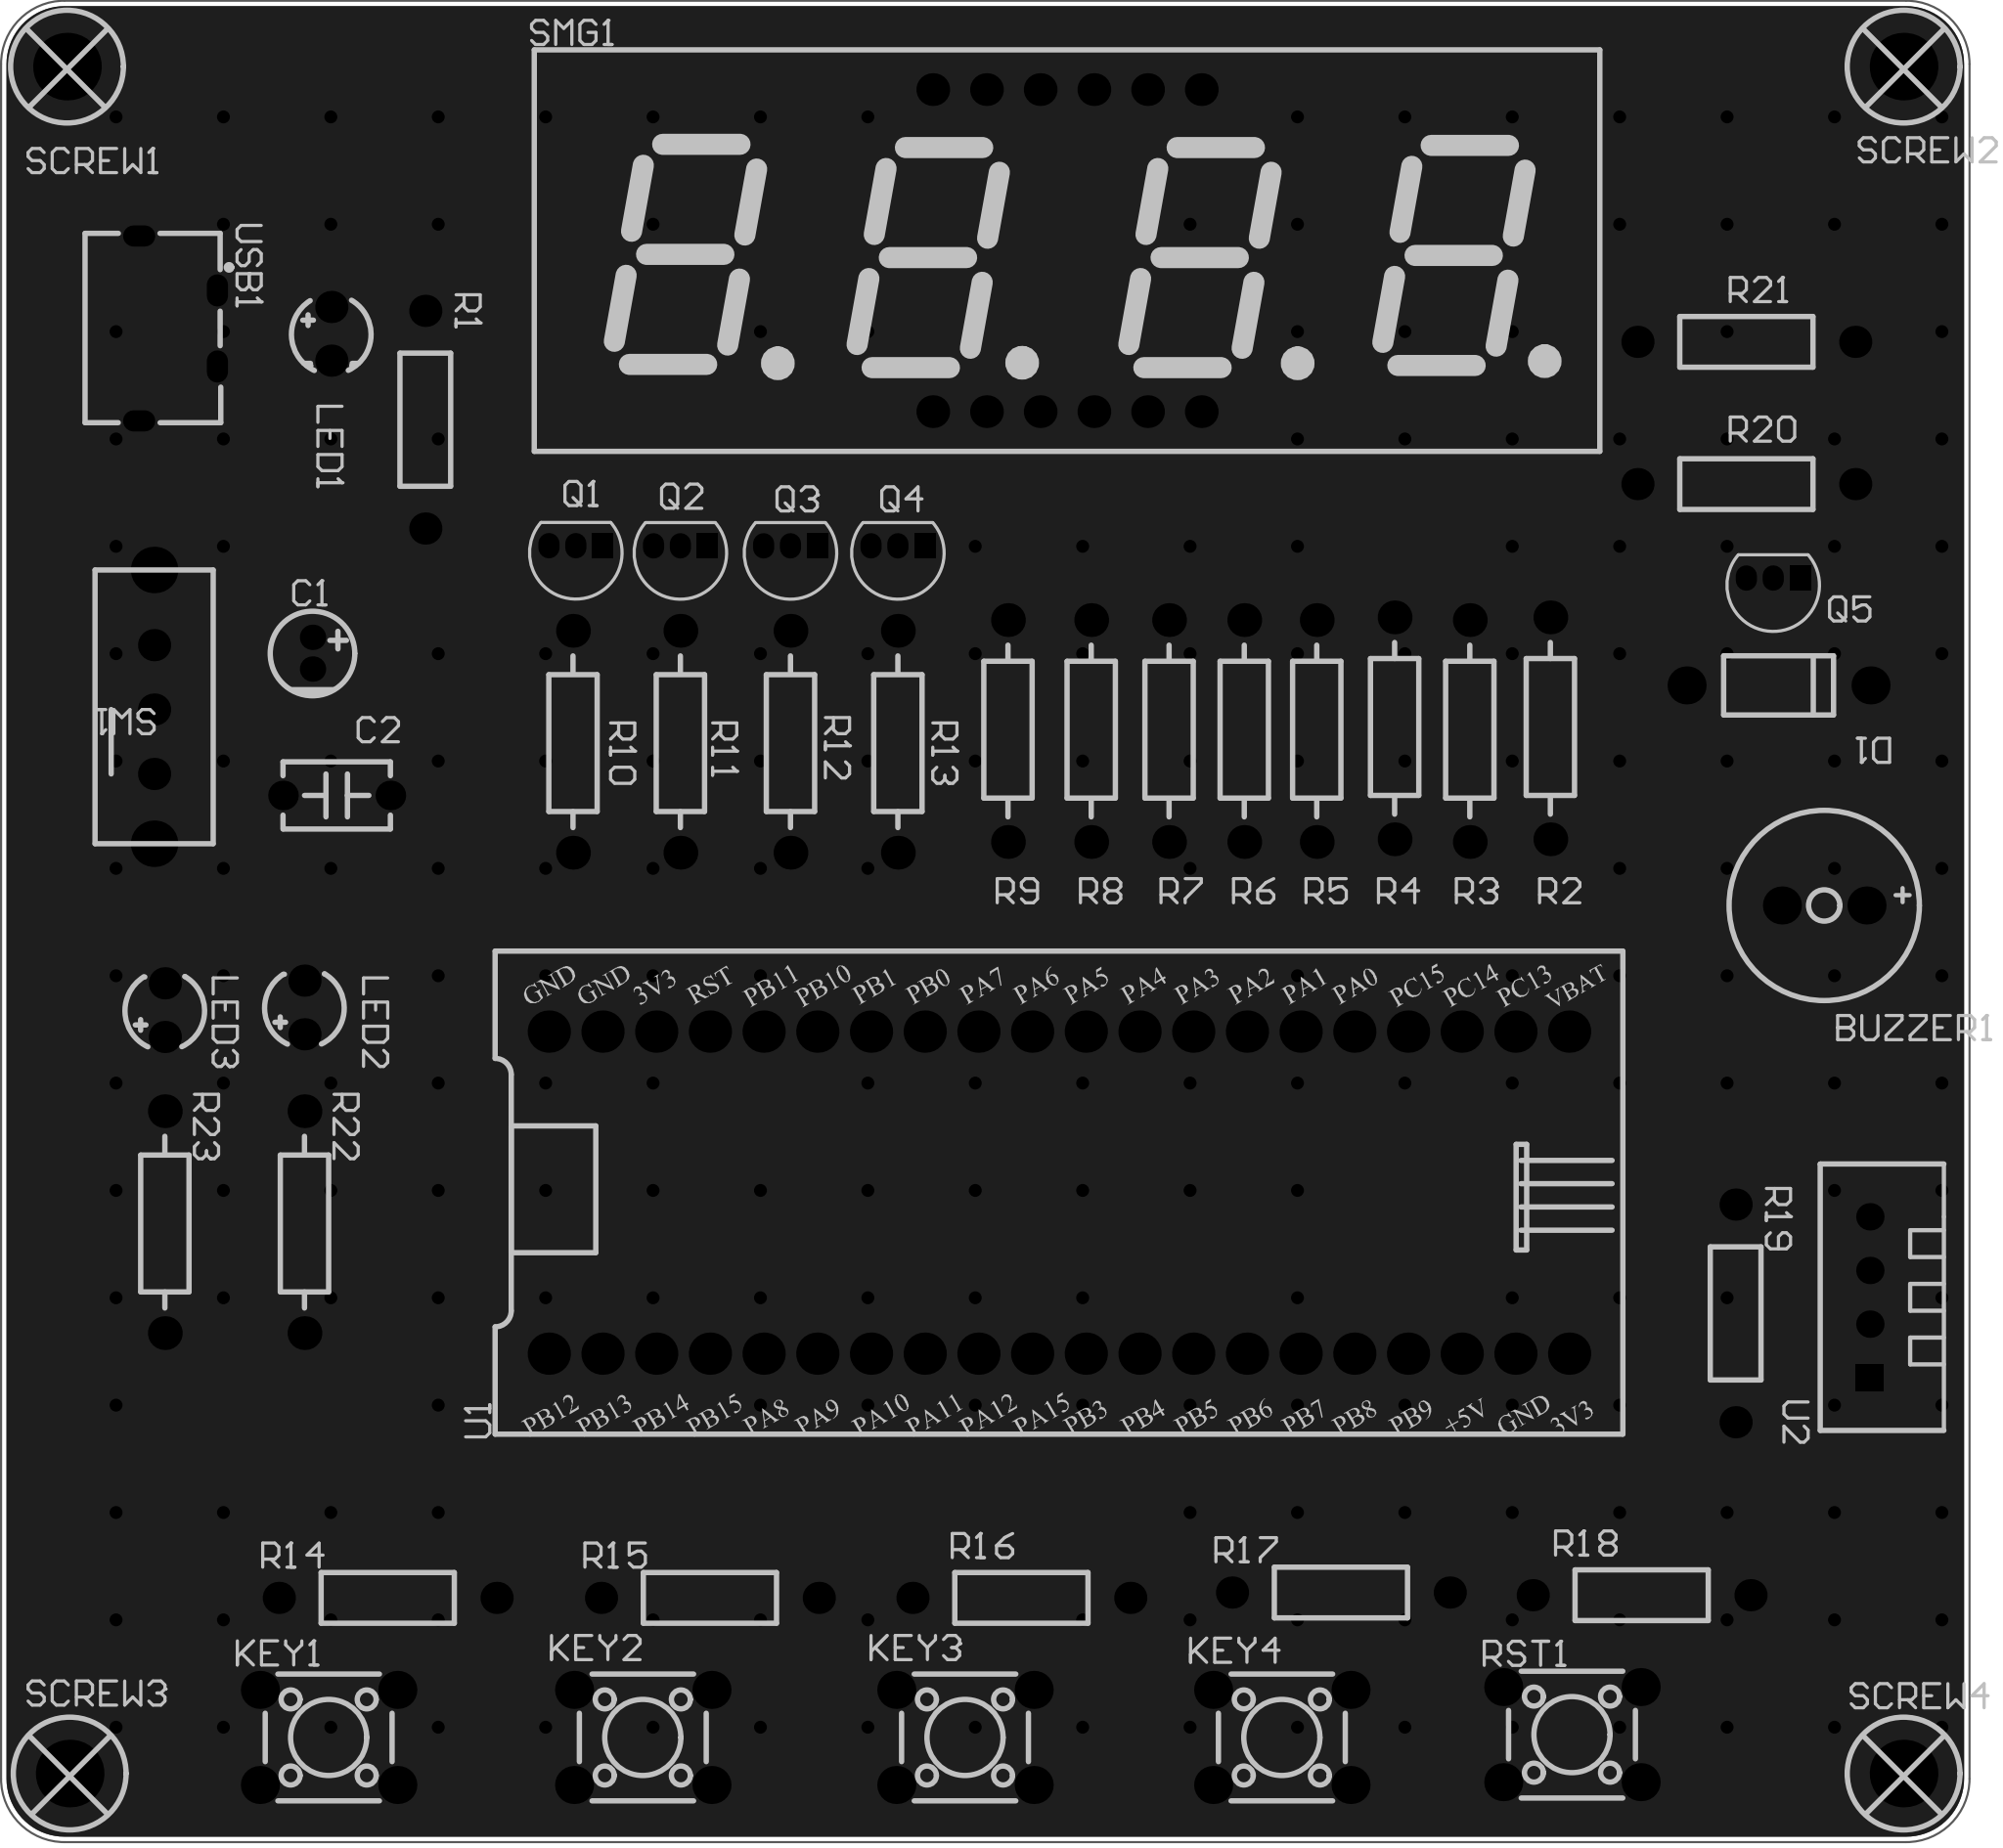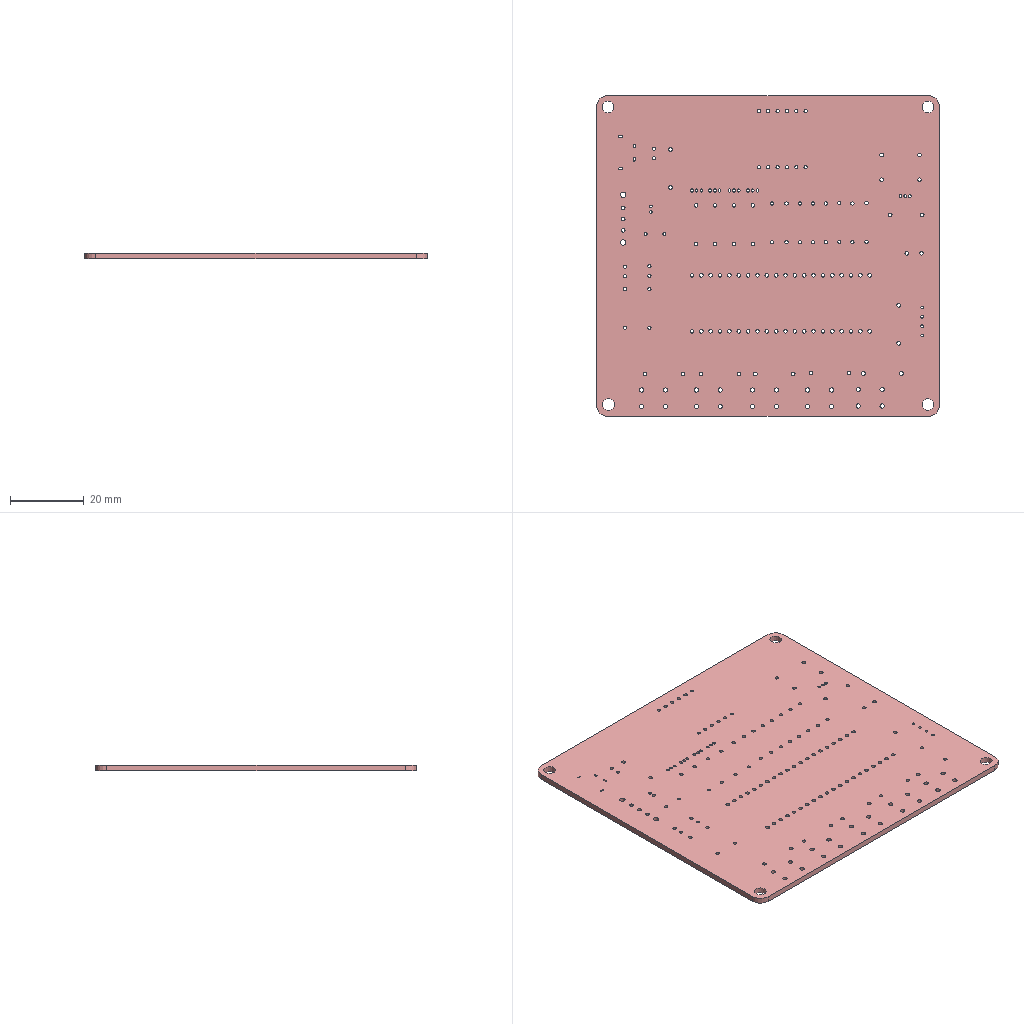Circuit board layout | Altium Designer | box 93.1 x 87.1 x 1.6 mm
Layer stack:
# Altium Designer layer stack of  (unit mm; dielectric type: 0 none, 1 core, 2 prepreg, 3 surface material)
index,name,kind,layer,copper_thickness_mm,dielectric_type,dielectric_thickness_mm,dielectric_material,dielectric_constant
0,Top Paste Mask Layer,other,,,,,,
1,Top Silkscreen Layer,other,,,,,,
2,Top Solder Mask Layer,dielectric,,,3,0.01,,3.3
3,Top Layer,copper,Top Layer,0.035,,,,
4,Dielectric1,dielectric,,,3,1.51,FR4,4.5
5,Bottom Layer,copper,Bottom Layer,0.035,,,,
6,Bottom Solder Mask Layer,dielectric,,,3,0.01,,3.3
7,Bottom Silkscreen Layer,other,,,,,,
8,Bottom Paste Mask Layer,other,,,,,,
# drill layer pairs: low layer,high layer
drill_pair,Top Layer,Bottom Layer
Part placement:
Designator,Comment,Layer,Footprint,Center-X(mm),Center-Y(mm),Rotation
BUZZER1,2.7kHz,TopLayer,BUZ-TH_BD9.0-P4.00-D0.6-FD,173.99,133.604,180
C1,10uF,TopLayer,CAP-TH_BD4.0-P1.50-D0.8-FD,102.489,145.542,270
C2,100nF,TopLayer,CAP-TH_L5.0-W2.5-P5.08-D0.7,103.632,138.811,180
D1,1N5819,TopLayer,DO-41_BD2.4-L4.7-P8.70-D0.9-RD,171.831,144.018,180
KEY1,TS-1002-07026,TopLayer,SW-TH_4P-L6.0-W6.0-P4.50-LS6.5,103.251,94.234,0
KEY2,TS-1002-07026,TopLayer,SW-TH_4P-L6.0-W6.0-P4.50-LS6.5,118.11,94.234,0
KEY3,TS-1002-07026,TopLayer,SW-TH_4P-L6.0-W6.0-P4.50-LS6.5,133.35,94.234,0
KEY4,TS-1002-07026,TopLayer,SW-TH_4P-L6.0-W6.0-P4.50-LS6.5,148.336,94.234,0
LED1,XL-302SURD,TopLayer,LED-TH_BD3.8-P2.54-RD,103.378,160.655,90
LED2,XL-302UGD,TopLayer,LED-TH_BD3.8-P2.54-FD_GREEN,102.108,128.778,90
LED3,XL-302UGD,TopLayer,LED-TH_BD3.8-P2.54-FD_GREEN,95.504,128.651,90
Q1,S8050,TopLayer,TO-92-3_L4.5-W3.5-P1.27-L,114.942,150.629,180
Q2,S8050,TopLayer,TO-92-3_L4.5-W3.5-P1.27-L,119.888,150.622,180
Q3,S8050,TopLayer,TO-92-3_L4.5-W3.5-P1.27-L,125.095,150.622,180
Q4,S8050,TopLayer,TO-92-3_L4.5-W3.5-P1.27-L,130.175,150.622,180
Q5,S8050,TopLayer,TO-92-3_L4.5-W3.5-P1.27-L,171.577,149.098,180
R1,10kΩ,TopLayer,RES-TH_BD2.4-L6.3-P10.30-D0.6,107.823,156.591,270
R2,330Ω,TopLayer,RES-TH_BD2.2-L6.5-P10.50-D0.6,161.036,141.986,90
R3,330Ω,TopLayer,RES-TH_BD2.2-L6.5-P10.50-D0.6,157.226,141.859,90
R4,330Ω,TopLayer,RES-TH_BD2.2-L6.5-P10.50-D0.6,153.67,141.986,90
R5,330Ω,TopLayer,RES-TH_BD2.2-L6.5-P10.50-D0.6,149.987,141.859,90
R6,330Ω,TopLayer,RES-TH_BD2.2-L6.5-P10.50-D0.6,146.558,141.859,90
R7,330Ω,TopLayer,RES-TH_BD2.2-L6.5-P10.50-D0.6,143.002,141.859,90
R8,330Ω,TopLayer,RES-TH_BD2.2-L6.5-P10.50-D0.6,139.319,141.859,90
R9,330Ω,TopLayer,RES-TH_BD2.2-L6.5-P10.50-D0.6,135.382,141.859,90
R10,1kΩ,TopLayer,RES-TH_BD2.2-L6.5-P10.50-D0.6,114.808,141.351,270
R11,1kΩ,TopLayer,RES-TH_BD2.2-L6.5-P10.50-D0.6,119.888,141.351,270
R12,1kΩ,TopLayer,RES-TH_BD2.2-L6.5-P10.50-D0.6,125.095,141.351,270
R13,1kΩ,TopLayer,RES-TH_BD2.2-L6.5-P10.50-D0.6,130.175,141.351,270
R14,10kΩ,TopLayer,RES-TH_BD2.4-L6.3-P10.30-D0.6,106.045,100.838,0
R15,10kΩ,TopLayer,RES-TH_BD2.4-L6.3-P10.30-D0.6,121.285,100.838,0
R16,10kΩ,TopLayer,RES-TH_BD2.4-L6.3-P10.30-D0.6,136.017,100.838,180
R17,10kΩ,TopLayer,RES-TH_BD2.4-L6.3-P10.30-D0.6,151.13,101.092,0
R18,10kΩ,TopLayer,RES-TH_BD2.4-L6.3-P10.30-D0.6,165.354,100.965,180
R19,10kΩ,TopLayer,RES-TH_BD2.4-L6.3-P10.30-D0.6,169.799,114.3,270
R20,10kΩ,TopLayer,RES-TH_BD2.4-L6.3-P10.30-D0.6,170.307,153.543,180
R21,10kΩ,TopLayer,RES-TH_BD2.4-L6.3-P10.30-D0.6,170.307,160.274,0
R22,1kΩ,TopLayer,RES-TH_BD2.2-L6.5-P10.50-D0.6,102.108,118.618,270
R23,1kΩ,TopLayer,RES-TH_BD2.2-L6.5-P10.50-D0.6,95.504,118.618,270
RST1,TS-1002-07026,TopLayer,SW-TH_4P-L6.0-W6.0-P4.50-LS6.5,162.059,94.368,0
SCREW1,,TopLayer,M3螺丝,90.876,173.298,0
SCREW2,,TopLayer,M3螺丝,177.744,173.298,0
SCREW3,,TopLayer,M3螺丝,91.002,92.526,0
SCREW4,,TopLayer,M3螺丝,177.744,92.526,0
SMG1,,TopLayer,LED-SEG-TH_FJ5461AH,138.176,164.592,0
SW1,SK-12E12-G5,TopLayer,SW-TH_SK-12E12-G5,94.996,143.002,180
U1,,TopLayer,GD32E230C8T6最小系统,137.795,120.015,90
U2,DHT11,TopLayer,SENSOR-TH_DHT11,176.149,115.062,90
USB1,KH-TYPE-C-2P,TopLayer,USB-SMD_KH-TYPE-C-2P,96.139,160.909,270
Pad and via stacks:
# Altium Designer via and pad stacks of  (unit mm). Each distinct definition once, with the count of objects using it.
# via: kind,start_layer,end_layer,hole_mm,diameter_mm,mode(0 simple;1 top-mid-bottom;2 full stack),diameter_per_layer,count,example_net
# pad: kind,layer,hole_mm,hole_type(0 round;1 square;2 slot),plating,top_size,top_shape(1 round;2 rect;3 octagon;9 rounded rect),mid_size,bottom_size,mode,footprint,size_per_layer,count,example
pad,Multi-Layer,1,0,plated,1.8x1.8,1,1.8x1.8,1.8x1.8,0,BUZ-TH_BD9.0-P4.00-D0.6-FD,,2,BUZZER1.1
pad,Multi-Layer,0.8,0,plated,1.2x1.2,1,1.2x1.2,1.2x1.2,0,CAP-TH_BD4.0-P1.50-D0.8-FD,,2,C1.2
pad,Multi-Layer,0.8,0,plated,1.4x1.4,1,1.4x1.4,1.4x1.4,0,CAP-TH_L5.0-W2.5-P5.08-D0.7,,2,C2.1
pad,Multi-Layer,1,0,plated,1.8x1.8,1,1.8x1.8,1.8x1.8,0,DO-41_BD2.4-L4.7-P8.70-D0.9-RD,,2,D1.1
pad,Multi-Layer,1.2,0,plated,1.8x1.8,1,1.8x1.8,1.8x1.8,0,SW-TH_4P-L6.0-W6.0-P4.50-LS6.5,,20,KEY1.1
pad,Multi-Layer,0.9,0,plated,1.524x1.524,1,1.524x1.524,1.524x1.524,0,LED-TH_BD3.8-P2.54-RD,,2,LED1.2
pad,Multi-Layer,0.9,0,plated,1.524x1.524,1,1.524x1.524,1.524x1.524,0,LED-TH_BD3.8-P2.54-FD_GREEN,,4,LED2.1
pad,Multi-Layer,0.7,2,plated,1x1.2,2,1x1.2,1x1.2,0,TO-92-3_L4.5-W3.5-P1.27-L,,5,Q1.1
pad,Multi-Layer,0.7,2,plated,1x1.2,1,1x1.2,1x1.2,0,TO-92-3_L4.5-W3.5-P1.27-L,,10,Q1.2
pad,Multi-Layer,1,0,plated,1.524x1.524,1,1.524x1.524,1.524x1.524,0,RES-TH_BD2.4-L6.3-P10.30-D0.6,,18,R1.1
pad,Multi-Layer,0.9144,0,plated,1.6x1.6,1,1.6x1.6,1.6x1.6,0,RES-TH_BD2.2-L6.5-P10.50-D0.6,,28,R2.1
pad,Multi-Layer,3.2,0,plated,3.2x3.2,1,3.2x3.2,3.2x3.2,0,M3\u00C2\u00DD\u00CB\u00BF,,4,SCREW1.1
pad,Multi-Layer,0.9,0,plated,1.55x1.55,1,1.55x1.55,1.55x1.55,0,LED-SEG-TH_FJ5461AH,,12,SMG1.4
pad,Multi-Layer,1,0,plated,1.524x1.524,1,1.524x1.524,1.524x1.524,0,SW-TH_SK-12E12-G5,,3,SW1.2
pad,Multi-Layer,1.5,0,plated,2.2x2.2,1,2.2x2.2,2.2x2.2,0,SW-TH_SK-12E12-G5,,2,SW1.4
pad,Multi-Layer,1,0,plated,2x2,1,2x2,2x2,0,GD32E230C8T6\u00D7\u00EE\u00D0\u00A1\u00CF\u00B5\u00CD\u00B3,,40,U1.1
pad,Multi-Layer,0.7112,0,plated,1.295x1.295,2,1.295x1.295,1.295x1.295,0,SENSOR-TH_DHT11,,1,U2.1
pad,Multi-Layer,0.7112,0,plated,1.295x1.295,1,1.295x1.295,1.295x1.295,0,SENSOR-TH_DHT11,,3,U2.2
pad,Multi-Layer,0.45,2,plated,1x1.524,1,1x1.524,1x1.524,0,USB-SMD_KH-TYPE-C-2P,,2,USB1.1
pad,Multi-Layer,0.5,2,plated,1x1.524,1,1x1.524,1x1.524,0,USB-SMD_KH-TYPE-C-2P,,2,USB1.3
via,Top Layer,Bottom Layer,0.3048,0.61,0,,222,GND
Copper pours:
name,layer,net,type(0 solid;1 hatched;2 none)
Top Layer-GND,Top Layer,GND,0
Bottom Layer-GND,Bottom Layer,GND,0
Design rules, without the lines most boards share:
# Altium Designer design rules of  (exported by Altium Designer, unit mm)
# columns: name | kind | enabled | priority | scope1 | scope2 | descriptor | typed fields (field=value)
PWR | 2 | enabled | 2 | (InNet('+5V') OR InNet('BUZZER') OR InNet('DIG1') OR InNet('DIG2') OR InNet('DIG3') OR InNet('DIG4') OR InNet('VCC')) | All | Width Constraint (Min=10mil) (Max=100mil) (Preferred=20mil) ((InNet('+5V') OR InNet('BUZZER') OR InNet('DIG1') OR InNet('DIG2') OR InNet('DIG3') OR InNet('DIG4') OR InNet('VCC'))) |
copperThickness1oz_2 | 2 | enabled | 3 | All | All | Width Constraint (Min=10mil) (Max=100mil) (Preferred=10mil) (All) |
viaSize | 11 | enabled | 1 | All | All | Routing Via (MinHoleWidth=12mil) (MaxHoleWidth=248.031mil) (PreferredHoleWidth=12.008mil) (MinWidth=24mil) (MaxWidth=393.701mil) (PreferedWidth=24.016mil) (All) | via_min_hole=0.3048 via_max_hole=6.3 via_preferred_diameter=0.61 via_preferred_hole=0.305